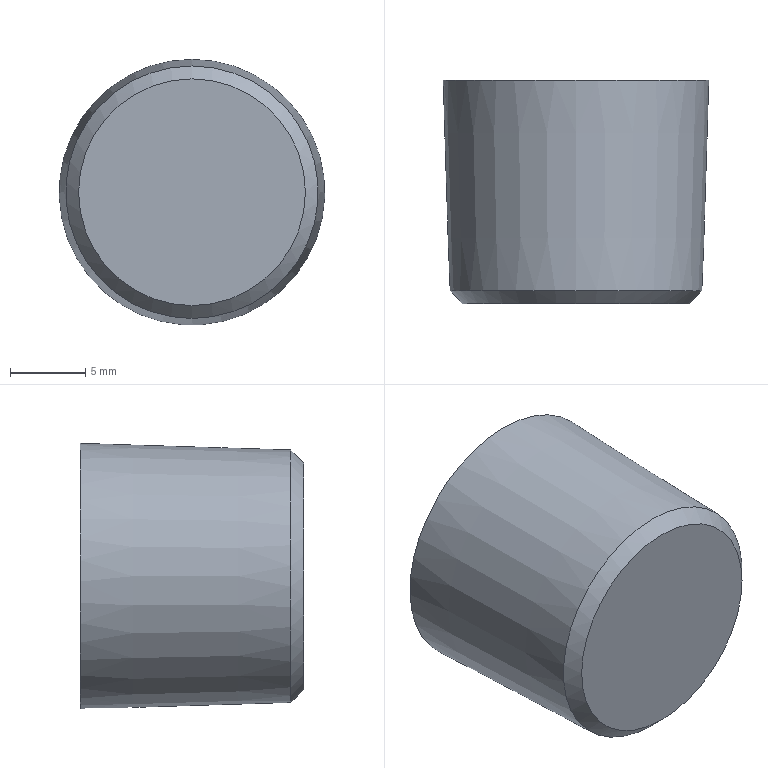Part | STEP file | solid 16 | 1 solid | 35 faces | box 17.662 x 14.856 x 17.662 mm | volume 2886 mm3 | plane 21 | other 12 | cone 2